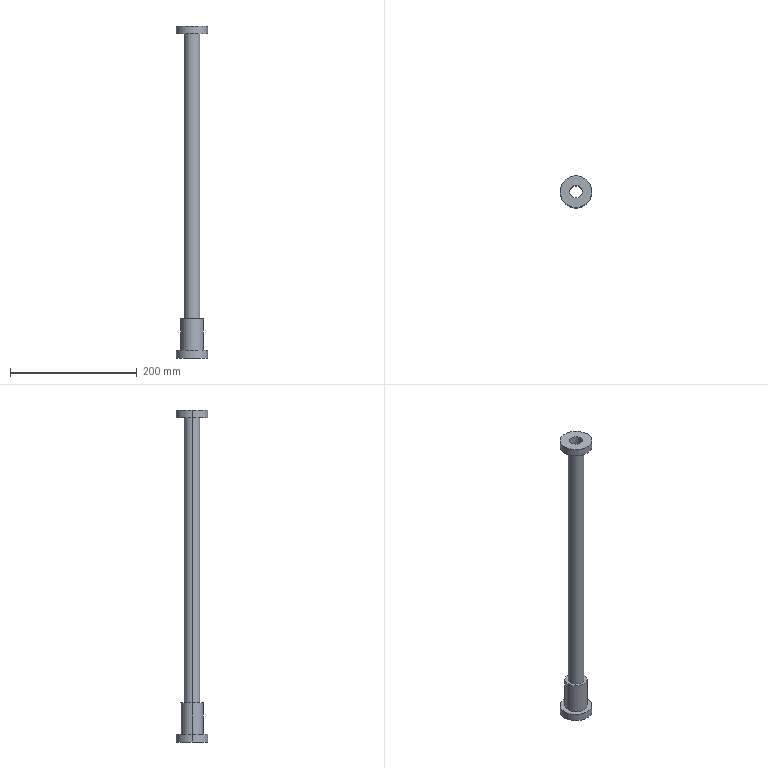Part | SolidWorks | features ICE 4, Extrusion 1 | 1 solid | 15 faces | box 50 x 50 x 524 mm | volume 151503 mm3 | cylinder 10 | plane 5 | commonest cylinder face diameters 50 x4 20 x2 25 x2 35 x2
STEP:
#1=CARTESIAN_POINT('',(-10.,0.,-62.));
#2=VERTEX_POINT('',#1);
#3=CARTESIAN_POINT('',(10.,0.,-62.));
#4=VERTEX_POINT('',#3);
#5=CARTESIAN_POINT('',(0.,0.,-62.));
#6=DIRECTION('',(0.,0.,1.));
#7=DIRECTION('',(1.,0.,0.));
#8=AXIS2_PLACEMENT_3D('',#5,#6,#7);
#9=CIRCLE('',#8,10.);
#10=EDGE_CURVE('',#2,#4,#9,.T.);
#11=ORIENTED_EDGE('',*,*,#10,.F.);
#12=CARTESIAN_POINT('',(-10.,0.,462.));
#13=VERTEX_POINT('',#12);
#14=CARTESIAN_POINT('',(-10.,0.,-62.));
#15=DIRECTION('',(0.,0.,1.));
#16=VECTOR('',#15,1000.);
#17=LINE('',#14,#16);
#18=EDGE_CURVE('',#2,#13,#17,.T.);
#19=ORIENTED_EDGE('',*,*,#18,.T.);
#20=CARTESIAN_POINT('',(10.,0.,462.));
#21=VERTEX_POINT('',#20);
#22=CARTESIAN_POINT('',(0.,0.,462.));
#23=DIRECTION('',(0.,0.,1.));
#24=DIRECTION('',(1.,0.,0.));
#25=AXIS2_PLACEMENT_3D('',#22,#23,#24);
#26=CIRCLE('',#25,10.);
#27=EDGE_CURVE('',#13,#21,#26,.T.);
#28=ORIENTED_EDGE('',*,*,#27,.T.);
#29=CARTESIAN_POINT('',(10.,0.,-62.));
#30=DIRECTION('',(0.,0.,1.));
#31=VECTOR('',#30,1000.);
#32=LINE('',#29,#31);
#33=EDGE_CURVE('',#4,#21,#32,.T.);
#34=ORIENTED_EDGE('',*,*,#33,.F.);
#35=EDGE_LOOP('',(#11,#19,#28,#34));
#36=FACE_OUTER_BOUND('',#35,.T.);
#37=CARTESIAN_POINT('',(0.,0.,-62.));
#38=DIRECTION('',(0.,0.,1.));
#39=DIRECTION('',(1.,0.,0.));
#40=AXIS2_PLACEMENT_3D('',#37,#38,#39);
#41=CYLINDRICAL_SURFACE('',#40,10.);
#42=ADVANCED_FACE('',(#36),#41,.F.);
#43=CARTESIAN_POINT('',(25.,0.,462.));
#44=VERTEX_POINT('',#43);
#45=CARTESIAN_POINT('',(-25.,0.,462.));
#46=VERTEX_POINT('',#45);
#47=CARTESIAN_POINT('',(0.,0.,462.));
#48=DIRECTION('',(0.,0.,1.));
#49=DIRECTION('',(1.,0.,0.));
#50=AXIS2_PLACEMENT_3D('',#47,#48,#49);
#51=CIRCLE('',#50,25.);
#52=EDGE_CURVE('',#44,#46,#51,.T.);
#53=ORIENTED_EDGE('',*,*,#52,.F.);
#54=CARTESIAN_POINT('',(25.,0.,450.));
#55=VERTEX_POINT('',#54);
#56=CARTESIAN_POINT('',(25.,0.,462.));
#57=DIRECTION('',(0.,0.,-1.));
#58=VECTOR('',#57,1000.);
#59=LINE('',#56,#58);
#60=EDGE_CURVE('',#44,#55,#59,.T.);
#61=ORIENTED_EDGE('',*,*,#60,.T.);
#62=CARTESIAN_POINT('',(-25.,0.,450.));
#63=VERTEX_POINT('',#62);
#64=CARTESIAN_POINT('',(0.,0.,450.));
#65=DIRECTION('',(0.,0.,1.));
#66=DIRECTION('',(1.,0.,0.));
#67=AXIS2_PLACEMENT_3D('',#64,#65,#66);
#68=CIRCLE('',#67,25.);
#69=EDGE_CURVE('',#55,#63,#68,.T.);
#70=ORIENTED_EDGE('',*,*,#69,.T.);
#71=CARTESIAN_POINT('',(-25.,0.,462.));
#72=DIRECTION('',(0.,0.,-1.));
#73=VECTOR('',#72,1000.);
#74=LINE('',#71,#73);
#75=EDGE_CURVE('',#46,#63,#74,.T.);
#76=ORIENTED_EDGE('',*,*,#75,.F.);
#77=EDGE_LOOP('',(#53,#61,#70,#76));
#78=FACE_OUTER_BOUND('',#77,.T.);
#79=CARTESIAN_POINT('',(0.,0.,462.));
#80=DIRECTION('',(0.,0.,-1.));
#81=DIRECTION('',(-1.,0.,0.));
#82=AXIS2_PLACEMENT_3D('',#79,#80,#81);
#83=CYLINDRICAL_SURFACE('',#82,25.);
#84=ADVANCED_FACE('',(#78),#83,.T.);
#85=CARTESIAN_POINT('',(-25.,0.,-62.));
#86=VERTEX_POINT('',#85);
#87=CARTESIAN_POINT('',(25.,0.,-62.));
#88=VERTEX_POINT('',#87);
#89=CARTESIAN_POINT('',(0.,0.,-62.));
#90=DIRECTION('',(0.,0.,-1.));
#91=DIRECTION('',(-1.,0.,0.));
#92=AXIS2_PLACEMENT_3D('',#89,#90,#91);
#93=CIRCLE('',#92,25.);
#94=EDGE_CURVE('',#86,#88,#93,.T.);
#95=ORIENTED_EDGE('',*,*,#94,.F.);
#96=CARTESIAN_POINT('',(-25.,0.,-50.));
#97=VERTEX_POINT('',#96);
#98=CARTESIAN_POINT('',(-25.,0.,-62.));
#99=DIRECTION('',(0.,0.,1.));
#100=VECTOR('',#99,1000.);
#101=LINE('',#98,#100);
#102=EDGE_CURVE('',#86,#97,#101,.T.);
#103=ORIENTED_EDGE('',*,*,#102,.T.);
#104=CARTESIAN_POINT('',(25.,0.,-50.));
#105=VERTEX_POINT('',#104);
#106=CARTESIAN_POINT('',(0.,0.,-50.));
#107=DIRECTION('',(0.,0.,-1.));
#108=DIRECTION('',(-1.,0.,0.));
#109=AXIS2_PLACEMENT_3D('',#106,#107,#108);
#110=CIRCLE('',#109,25.);
#111=EDGE_CURVE('',#97,#105,#110,.T.);
#112=ORIENTED_EDGE('',*,*,#111,.T.);
#113=CARTESIAN_POINT('',(25.,0.,-62.));
#114=DIRECTION('',(0.,0.,1.));
#115=VECTOR('',#114,1000.);
#116=LINE('',#113,#115);
#117=EDGE_CURVE('',#88,#105,#116,.T.);
#118=ORIENTED_EDGE('',*,*,#117,.F.);
#119=EDGE_LOOP('',(#95,#103,#112,#118));
#120=FACE_OUTER_BOUND('',#119,.T.);
#121=CARTESIAN_POINT('',(0.,0.,-62.));
#122=DIRECTION('',(0.,0.,1.));
#123=DIRECTION('',(1.,0.,0.));
#124=AXIS2_PLACEMENT_3D('',#121,#122,#123);
#125=CYLINDRICAL_SURFACE('',#124,25.);
#126=ADVANCED_FACE('',(#120),#125,.T.);
#127=CARTESIAN_POINT('',(-17.5,0.,-50.));
#128=VERTEX_POINT('',#127);
#129=CARTESIAN_POINT('',(17.5,0.,-50.));
#130=VERTEX_POINT('',#129);
#131=CARTESIAN_POINT('',(0.,0.,-50.));
#132=DIRECTION('',(0.,0.,-1.));
#133=DIRECTION('',(-1.,0.,0.));
#134=AXIS2_PLACEMENT_3D('',#131,#132,#133);
#135=CIRCLE('',#134,17.5);
#136=EDGE_CURVE('',#128,#130,#135,.T.);
#137=ORIENTED_EDGE('',*,*,#136,.F.);
#138=CARTESIAN_POINT('',(-17.5,0.,0.));
#139=VERTEX_POINT('',#138);
#140=CARTESIAN_POINT('',(-17.5,0.,-50.));
#141=DIRECTION('',(0.,0.,1.));
#142=VECTOR('',#141,1000.);
#143=LINE('',#140,#142);
#144=EDGE_CURVE('',#128,#139,#143,.T.);
#145=ORIENTED_EDGE('',*,*,#144,.T.);
#146=CARTESIAN_POINT('',(17.5,0.,0.));
#147=VERTEX_POINT('',#146);
#148=CARTESIAN_POINT('',(0.,0.,0.));
#149=DIRECTION('',(0.,0.,-1.));
#150=DIRECTION('',(-1.,0.,0.));
#151=AXIS2_PLACEMENT_3D('',#148,#149,#150);
#152=CIRCLE('',#151,17.5);
#153=EDGE_CURVE('',#139,#147,#152,.T.);
#154=ORIENTED_EDGE('',*,*,#153,.T.);
#155=CARTESIAN_POINT('',(17.5,0.,-50.));
#156=DIRECTION('',(0.,0.,1.));
#157=VECTOR('',#156,1000.);
#158=LINE('',#155,#157);
#159=EDGE_CURVE('',#130,#147,#158,.T.);
#160=ORIENTED_EDGE('',*,*,#159,.F.);
#161=EDGE_LOOP('',(#137,#145,#154,#160));
#162=FACE_OUTER_BOUND('',#161,.T.);
#163=CARTESIAN_POINT('',(0.,0.,-50.));
#164=DIRECTION('',(0.,0.,1.));
#165=DIRECTION('',(1.,0.,0.));
#166=AXIS2_PLACEMENT_3D('',#163,#164,#165);
#167=CYLINDRICAL_SURFACE('',#166,17.5);
#168=ADVANCED_FACE('',(#162),#167,.T.);
#169=CARTESIAN_POINT('',(12.5,0.,450.));
#170=VERTEX_POINT('',#169);
#171=CARTESIAN_POINT('',(-12.5,0.,450.));
#172=VERTEX_POINT('',#171);
#173=CARTESIAN_POINT('',(0.,0.,450.));
#174=DIRECTION('',(0.,0.,1.));
#175=DIRECTION('',(1.,0.,0.));
#176=AXIS2_PLACEMENT_3D('',#173,#174,#175);
#177=CIRCLE('',#176,12.5);
#178=EDGE_CURVE('',#170,#172,#177,.T.);
#179=ORIENTED_EDGE('',*,*,#178,.F.);
#180=CARTESIAN_POINT('',(12.5,0.,0.));
#181=VERTEX_POINT('',#180);
#182=CARTESIAN_POINT('',(12.5,0.,450.));
#183=DIRECTION('',(0.,0.,-1.));
#184=VECTOR('',#183,1000.);
#185=LINE('',#182,#184);
#186=EDGE_CURVE('',#170,#181,#185,.T.);
#187=ORIENTED_EDGE('',*,*,#186,.T.);
#188=CARTESIAN_POINT('',(-12.5,0.,0.));
#189=VERTEX_POINT('',#188);
#190=CARTESIAN_POINT('',(0.,0.,0.));
#191=DIRECTION('',(0.,0.,-1.));
#192=DIRECTION('',(-1.,0.,0.));
#193=AXIS2_PLACEMENT_3D('',#190,#191,#192);
#194=CIRCLE('',#193,12.5);
#195=EDGE_CURVE('',#189,#181,#194,.T.);
#196=ORIENTED_EDGE('',*,*,#195,.F.);
#197=CARTESIAN_POINT('',(-12.5,0.,450.));
#198=DIRECTION('',(0.,0.,-1.));
#199=VECTOR('',#198,1000.);
#200=LINE('',#197,#199);
#201=EDGE_CURVE('',#172,#189,#200,.T.);
#202=ORIENTED_EDGE('',*,*,#201,.F.);
#203=EDGE_LOOP('',(#179,#187,#196,#202));
#204=FACE_OUTER_BOUND('',#203,.T.);
#205=CARTESIAN_POINT('',(0.,0.,450.));
#206=DIRECTION('',(0.,0.,-1.));
#207=DIRECTION('',(-1.,0.,0.));
#208=AXIS2_PLACEMENT_3D('',#205,#206,#207);
#209=CYLINDRICAL_SURFACE('',#208,12.5);
#210=ADVANCED_FACE('',(#204),#209,.T.);
#211=ORIENTED_EDGE('',*,*,#186,.F.);
#212=CARTESIAN_POINT('',(0.,0.,450.));
#213=DIRECTION('',(0.,0.,1.));
#214=DIRECTION('',(1.,0.,0.));
#215=AXIS2_PLACEMENT_3D('',#212,#213,#214);
#216=CIRCLE('',#215,12.5);
#217=EDGE_CURVE('',#172,#170,#216,.T.);
#218=ORIENTED_EDGE('',*,*,#217,.F.);
#219=ORIENTED_EDGE('',*,*,#201,.T.);
#220=CARTESIAN_POINT('',(0.,0.,0.));
#221=DIRECTION('',(0.,0.,-1.));
#222=DIRECTION('',(-1.,0.,0.));
#223=AXIS2_PLACEMENT_3D('',#220,#221,#222);
#224=CIRCLE('',#223,12.5);
#225=EDGE_CURVE('',#181,#189,#224,.T.);
#226=ORIENTED_EDGE('',*,*,#225,.F.);
#227=EDGE_LOOP('',(#211,#218,#219,#226));
#228=FACE_OUTER_BOUND('',#227,.T.);
#229=CARTESIAN_POINT('',(0.,0.,450.));
#230=DIRECTION('',(0.,0.,-1.));
#231=DIRECTION('',(-1.,0.,0.));
#232=AXIS2_PLACEMENT_3D('',#229,#230,#231);
#233=CYLINDRICAL_SURFACE('',#232,12.5);
#234=ADVANCED_FACE('',(#228),#233,.T.);
#235=ORIENTED_EDGE('',*,*,#144,.F.);
#236=CARTESIAN_POINT('',(0.,0.,-50.));
#237=DIRECTION('',(0.,0.,-1.));
#238=DIRECTION('',(-1.,0.,0.));
#239=AXIS2_PLACEMENT_3D('',#236,#237,#238);
#240=CIRCLE('',#239,17.5);
#241=EDGE_CURVE('',#130,#128,#240,.T.);
#242=ORIENTED_EDGE('',*,*,#241,.F.);
#243=ORIENTED_EDGE('',*,*,#159,.T.);
#244=CARTESIAN_POINT('',(0.,0.,0.));
#245=DIRECTION('',(0.,0.,-1.));
#246=DIRECTION('',(-1.,0.,0.));
#247=AXIS2_PLACEMENT_3D('',#244,#245,#246);
#248=CIRCLE('',#247,17.5);
#249=EDGE_CURVE('',#147,#139,#248,.T.);
#250=ORIENTED_EDGE('',*,*,#249,.T.);
#251=EDGE_LOOP('',(#235,#242,#243,#250));
#252=FACE_OUTER_BOUND('',#251,.T.);
#253=CARTESIAN_POINT('',(0.,0.,-50.));
#254=DIRECTION('',(0.,0.,1.));
#255=DIRECTION('',(1.,0.,0.));
#256=AXIS2_PLACEMENT_3D('',#253,#254,#255);
#257=CYLINDRICAL_SURFACE('',#256,17.5);
#258=ADVANCED_FACE('',(#252),#257,.T.);
#259=ORIENTED_EDGE('',*,*,#195,.T.);
#260=ORIENTED_EDGE('',*,*,#225,.T.);
#261=EDGE_LOOP('',(#259,#260));
#262=FACE_BOUND('',#261,.T.);
#263=ORIENTED_EDGE('',*,*,#249,.F.);
#264=ORIENTED_EDGE('',*,*,#153,.F.);
#265=EDGE_LOOP('',(#263,#264));
#266=FACE_OUTER_BOUND('',#265,.T.);
#267=CARTESIAN_POINT('',(0.,0.,0.));
#268=DIRECTION('',(0.,0.,-1.));
#269=DIRECTION('',(-1.,0.,0.));
#270=AXIS2_PLACEMENT_3D('',#267,#268,#269);
#271=PLANE('',#270);
#272=ADVANCED_FACE('',(#262,#266),#271,.F.);
#273=ORIENTED_EDGE('',*,*,#102,.F.);
#274=CARTESIAN_POINT('',(0.,0.,-62.));
#275=DIRECTION('',(0.,0.,-1.));
#276=DIRECTION('',(-1.,0.,0.));
#277=AXIS2_PLACEMENT_3D('',#274,#275,#276);
#278=CIRCLE('',#277,25.);
#279=EDGE_CURVE('',#88,#86,#278,.T.);
#280=ORIENTED_EDGE('',*,*,#279,.F.);
#281=ORIENTED_EDGE('',*,*,#117,.T.);
#282=CARTESIAN_POINT('',(0.,0.,-50.));
#283=DIRECTION('',(0.,0.,-1.));
#284=DIRECTION('',(-1.,0.,0.));
#285=AXIS2_PLACEMENT_3D('',#282,#283,#284);
#286=CIRCLE('',#285,25.);
#287=EDGE_CURVE('',#105,#97,#286,.T.);
#288=ORIENTED_EDGE('',*,*,#287,.T.);
#289=EDGE_LOOP('',(#273,#280,#281,#288));
#290=FACE_OUTER_BOUND('',#289,.T.);
#291=CARTESIAN_POINT('',(0.,0.,-62.));
#292=DIRECTION('',(0.,0.,1.));
#293=DIRECTION('',(1.,0.,0.));
#294=AXIS2_PLACEMENT_3D('',#291,#292,#293);
#295=CYLINDRICAL_SURFACE('',#294,25.);
#296=ADVANCED_FACE('',(#290),#295,.T.);
#297=CARTESIAN_POINT('',(0.,0.,-62.));
#298=DIRECTION('',(0.,0.,1.));
#299=DIRECTION('',(1.,0.,0.));
#300=AXIS2_PLACEMENT_3D('',#297,#298,#299);
#301=CIRCLE('',#300,10.);
#302=EDGE_CURVE('',#4,#2,#301,.T.);
#303=ORIENTED_EDGE('',*,*,#302,.T.);
#304=ORIENTED_EDGE('',*,*,#10,.T.);
#305=EDGE_LOOP('',(#303,#304));
#306=FACE_BOUND('',#305,.T.);
#307=ORIENTED_EDGE('',*,*,#279,.T.);
#308=ORIENTED_EDGE('',*,*,#94,.T.);
#309=EDGE_LOOP('',(#307,#308));
#310=FACE_OUTER_BOUND('',#309,.T.);
#311=CARTESIAN_POINT('',(0.,0.,-62.));
#312=DIRECTION('',(0.,0.,-1.));
#313=DIRECTION('',(-1.,0.,0.));
#314=AXIS2_PLACEMENT_3D('',#311,#312,#313);
#315=PLANE('',#314);
#316=ADVANCED_FACE('',(#306,#310),#315,.T.);
#317=ORIENTED_EDGE('',*,*,#241,.T.);
#318=ORIENTED_EDGE('',*,*,#136,.T.);
#319=EDGE_LOOP('',(#317,#318));
#320=FACE_BOUND('',#319,.T.);
#321=ORIENTED_EDGE('',*,*,#287,.F.);
#322=ORIENTED_EDGE('',*,*,#111,.F.);
#323=EDGE_LOOP('',(#321,#322));
#324=FACE_OUTER_BOUND('',#323,.T.);
#325=CARTESIAN_POINT('',(0.,0.,-50.));
#326=DIRECTION('',(0.,0.,-1.));
#327=DIRECTION('',(-1.,0.,0.));
#328=AXIS2_PLACEMENT_3D('',#325,#326,#327);
#329=PLANE('',#328);
#330=ADVANCED_FACE('',(#320,#324),#329,.F.);
#331=ORIENTED_EDGE('',*,*,#60,.F.);
#332=CARTESIAN_POINT('',(0.,0.,462.));
#333=DIRECTION('',(0.,0.,1.));
#334=DIRECTION('',(1.,0.,0.));
#335=AXIS2_PLACEMENT_3D('',#332,#333,#334);
#336=CIRCLE('',#335,25.);
#337=EDGE_CURVE('',#46,#44,#336,.T.);
#338=ORIENTED_EDGE('',*,*,#337,.F.);
#339=ORIENTED_EDGE('',*,*,#75,.T.);
#340=CARTESIAN_POINT('',(0.,0.,450.));
#341=DIRECTION('',(0.,0.,1.));
#342=DIRECTION('',(1.,0.,0.));
#343=AXIS2_PLACEMENT_3D('',#340,#341,#342);
#344=CIRCLE('',#343,25.);
#345=EDGE_CURVE('',#63,#55,#344,.T.);
#346=ORIENTED_EDGE('',*,*,#345,.T.);
#347=EDGE_LOOP('',(#331,#338,#339,#346));
#348=FACE_OUTER_BOUND('',#347,.T.);
#349=CARTESIAN_POINT('',(0.,0.,462.));
#350=DIRECTION('',(0.,0.,-1.));
#351=DIRECTION('',(-1.,0.,0.));
#352=AXIS2_PLACEMENT_3D('',#349,#350,#351);
#353=CYLINDRICAL_SURFACE('',#352,25.);
#354=ADVANCED_FACE('',(#348),#353,.T.);
#355=CARTESIAN_POINT('',(0.,0.,462.));
#356=DIRECTION('',(0.,0.,1.));
#357=DIRECTION('',(1.,0.,0.));
#358=AXIS2_PLACEMENT_3D('',#355,#356,#357);
#359=CIRCLE('',#358,10.);
#360=EDGE_CURVE('',#21,#13,#359,.T.);
#361=ORIENTED_EDGE('',*,*,#360,.F.);
#362=ORIENTED_EDGE('',*,*,#27,.F.);
#363=EDGE_LOOP('',(#361,#362));
#364=FACE_BOUND('',#363,.T.);
#365=ORIENTED_EDGE('',*,*,#337,.T.);
#366=ORIENTED_EDGE('',*,*,#52,.T.);
#367=EDGE_LOOP('',(#365,#366));
#368=FACE_OUTER_BOUND('',#367,.T.);
#369=CARTESIAN_POINT('',(0.,0.,462.));
#370=DIRECTION('',(0.,0.,1.));
#371=DIRECTION('',(1.,0.,0.));
#372=AXIS2_PLACEMENT_3D('',#369,#370,#371);
#373=PLANE('',#372);
#374=ADVANCED_FACE('',(#364,#368),#373,.T.);
#375=ORIENTED_EDGE('',*,*,#217,.T.);
#376=ORIENTED_EDGE('',*,*,#178,.T.);
#377=EDGE_LOOP('',(#375,#376));
#378=FACE_BOUND('',#377,.T.);
#379=ORIENTED_EDGE('',*,*,#345,.F.);
#380=ORIENTED_EDGE('',*,*,#69,.F.);
#381=EDGE_LOOP('',(#379,#380));
#382=FACE_OUTER_BOUND('',#381,.T.);
#383=CARTESIAN_POINT('',(0.,0.,450.));
#384=DIRECTION('',(0.,0.,1.));
#385=DIRECTION('',(1.,0.,0.));
#386=AXIS2_PLACEMENT_3D('',#383,#384,#385);
#387=PLANE('',#386);
#388=ADVANCED_FACE('',(#378,#382),#387,.F.);
#389=ORIENTED_EDGE('',*,*,#18,.F.);
#390=ORIENTED_EDGE('',*,*,#302,.F.);
#391=ORIENTED_EDGE('',*,*,#33,.T.);
#392=ORIENTED_EDGE('',*,*,#360,.T.);
#393=EDGE_LOOP('',(#389,#390,#391,#392));
#394=FACE_OUTER_BOUND('',#393,.T.);
#395=CARTESIAN_POINT('',(0.,0.,-62.));
#396=DIRECTION('',(0.,0.,1.));
#397=DIRECTION('',(1.,0.,0.));
#398=AXIS2_PLACEMENT_3D('',#395,#396,#397);
#399=CYLINDRICAL_SURFACE('',#398,10.);
#400=ADVANCED_FACE('',(#394),#399,.F.);
#401=CLOSED_SHELL('',(#42,#84,#126,#168,#210,#234,#258,#272,#296,#316,#330,#354,#374,#388,#400));
#402=MANIFOLD_SOLID_BREP('',#401);
#403=CARTESIAN_POINT('',(0.,0.,0.));
#404=DIRECTION('',(0.,0.,1.));
#405=DIRECTION('',(1.,0.,0.));
#406=AXIS2_PLACEMENT_3D('',#403,#404,#405);
#407=(LENGTH_UNIT()NAMED_UNIT(*)SI_UNIT(.MILLI.,.METRE.));
#408=UNCERTAINTY_MEASURE_WITH_UNIT(LENGTH_MEASURE(0.00001),#407,'','');
#409=(NAMED_UNIT(*)PLANE_ANGLE_UNIT()SI_UNIT($,.RADIAN.));
#410=(NAMED_UNIT(*)SI_UNIT($,.STERADIAN.)SOLID_ANGLE_UNIT());
#411=(GEOMETRIC_REPRESENTATION_CONTEXT(3)GLOBAL_UNCERTAINTY_ASSIGNED_CONTEXT((#408))GLOBAL_UNIT_ASSIGNED_CONTEXT((#407,#409,#410))REPRESENTATION_CONTEXT('',''));
#412=ADVANCED_BREP_SHAPE_REPRESENTATION('',(#402,#406),#411);